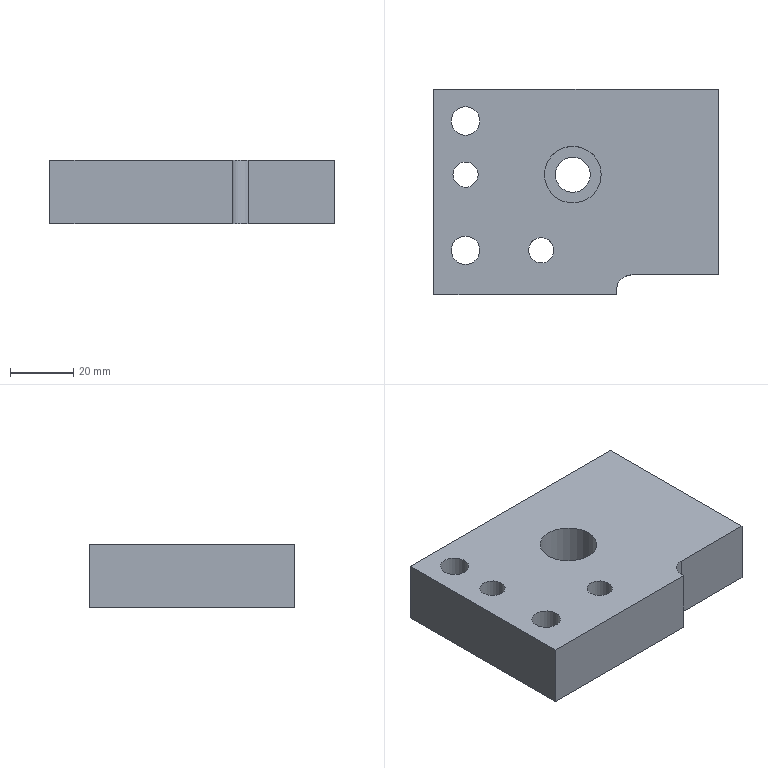Part | STEP file | 401_id30_x_t | 1 solid | 24 faces | box 90 x 65 x 20 mm | volume 101509 mm3 | plane 13 | cylinder 11 | commonest cylinder face diameters 10 x3 8 x2 9 x2 14 x2 11.1 x1 18 x1